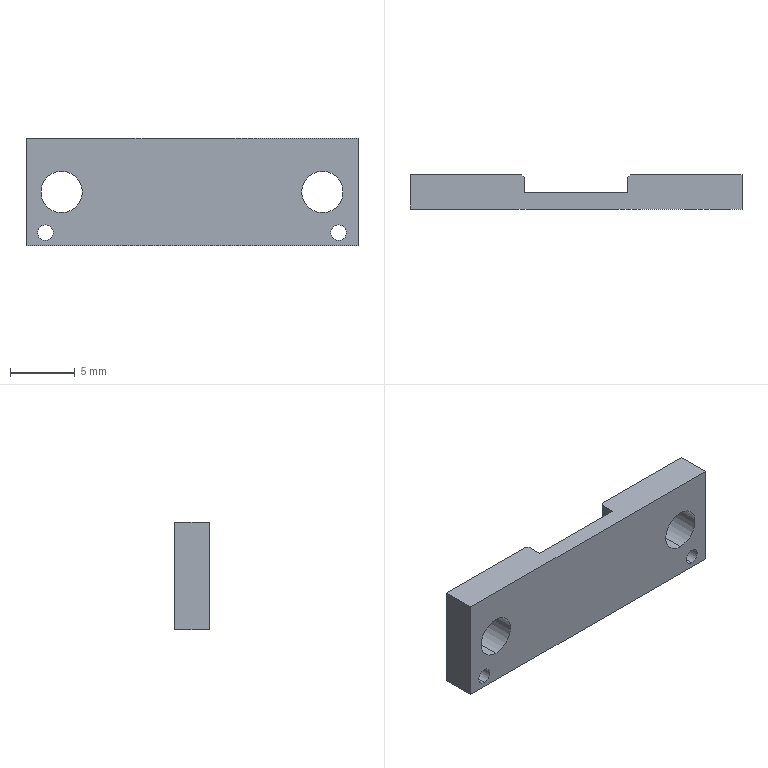Part | SolidWorks | features Chamfer 1, Extrusion 1, ICE 1 | 1 solid | 20 faces | box 25.7 x 2.65 x 8.3 mm | volume 426.68 mm3 | plane 12 | cylinder 8 | commonest cylinder face diameters 1.2 x4 3.2 x4
STEP:
#1=CARTESIAN_POINT('',(10.1,2.65,-1.6));
#2=VERTEX_POINT('',#1);
#3=CARTESIAN_POINT('',(10.1,2.65,1.6));
#4=VERTEX_POINT('',#3);
#5=CARTESIAN_POINT('',(10.1,2.65,0.));
#6=DIRECTION('',(0.,1.,0.));
#7=DIRECTION('',(0.,0.,-1.));
#8=AXIS2_PLACEMENT_3D('',#5,#6,#7);
#9=CIRCLE('',#8,1.6);
#10=EDGE_CURVE('',#2,#4,#9,.T.);
#11=ORIENTED_EDGE('',*,*,#10,.T.);
#12=CARTESIAN_POINT('',(10.1,0.,1.6));
#13=VERTEX_POINT('',#12);
#14=CARTESIAN_POINT('',(10.1,2.65,1.6));
#15=DIRECTION('',(0.,-1.,0.));
#16=VECTOR('',#15,1000.);
#17=LINE('',#14,#16);
#18=EDGE_CURVE('',#4,#13,#17,.T.);
#19=ORIENTED_EDGE('',*,*,#18,.T.);
#20=CARTESIAN_POINT('',(10.1,0.,-1.6));
#21=VERTEX_POINT('',#20);
#22=CARTESIAN_POINT('',(10.1,0.,0.));
#23=DIRECTION('',(0.,1.,0.));
#24=DIRECTION('',(0.,0.,-1.));
#25=AXIS2_PLACEMENT_3D('',#22,#23,#24);
#26=CIRCLE('',#25,1.6);
#27=EDGE_CURVE('',#21,#13,#26,.T.);
#28=ORIENTED_EDGE('',*,*,#27,.F.);
#29=CARTESIAN_POINT('',(10.1,2.65,-1.6));
#30=DIRECTION('',(0.,-1.,0.));
#31=VECTOR('',#30,1000.);
#32=LINE('',#29,#31);
#33=EDGE_CURVE('',#2,#21,#32,.T.);
#34=ORIENTED_EDGE('',*,*,#33,.F.);
#35=EDGE_LOOP('',(#11,#19,#28,#34));
#36=FACE_OUTER_BOUND('',#35,.T.);
#37=CARTESIAN_POINT('',(10.1,2.65,0.));
#38=DIRECTION('',(0.,-1.,0.));
#39=DIRECTION('',(0.,0.,-1.));
#40=AXIS2_PLACEMENT_3D('',#37,#38,#39);
#41=CYLINDRICAL_SURFACE('',#40,1.6);
#42=ADVANCED_FACE('',(#36),#41,.F.);
#43=CARTESIAN_POINT('',(11.35,2.65,-3.75));
#44=VERTEX_POINT('',#43);
#45=CARTESIAN_POINT('',(11.35,2.65,-2.55));
#46=VERTEX_POINT('',#45);
#47=CARTESIAN_POINT('',(11.35,2.65,-3.15));
#48=DIRECTION('',(0.,1.,0.));
#49=DIRECTION('',(0.,0.,-1.));
#50=AXIS2_PLACEMENT_3D('',#47,#48,#49);
#51=CIRCLE('',#50,0.6);
#52=EDGE_CURVE('',#44,#46,#51,.T.);
#53=ORIENTED_EDGE('',*,*,#52,.T.);
#54=CARTESIAN_POINT('',(11.35,0.,-2.55));
#55=VERTEX_POINT('',#54);
#56=CARTESIAN_POINT('',(11.35,2.65,-2.55));
#57=DIRECTION('',(0.,-1.,0.));
#58=VECTOR('',#57,1000.);
#59=LINE('',#56,#58);
#60=EDGE_CURVE('',#46,#55,#59,.T.);
#61=ORIENTED_EDGE('',*,*,#60,.T.);
#62=CARTESIAN_POINT('',(11.35,0.,-3.75));
#63=VERTEX_POINT('',#62);
#64=CARTESIAN_POINT('',(11.35,0.,-3.15));
#65=DIRECTION('',(0.,1.,0.));
#66=DIRECTION('',(0.,0.,-1.));
#67=AXIS2_PLACEMENT_3D('',#64,#65,#66);
#68=CIRCLE('',#67,0.6);
#69=EDGE_CURVE('',#63,#55,#68,.T.);
#70=ORIENTED_EDGE('',*,*,#69,.F.);
#71=CARTESIAN_POINT('',(11.35,2.65,-3.75));
#72=DIRECTION('',(0.,-1.,0.));
#73=VECTOR('',#72,1000.);
#74=LINE('',#71,#73);
#75=EDGE_CURVE('',#44,#63,#74,.T.);
#76=ORIENTED_EDGE('',*,*,#75,.F.);
#77=EDGE_LOOP('',(#53,#61,#70,#76));
#78=FACE_OUTER_BOUND('',#77,.T.);
#79=CARTESIAN_POINT('',(11.35,2.65,-3.15));
#80=DIRECTION('',(0.,-1.,0.));
#81=DIRECTION('',(0.,0.,-1.));
#82=AXIS2_PLACEMENT_3D('',#79,#80,#81);
#83=CYLINDRICAL_SURFACE('',#82,0.6);
#84=ADVANCED_FACE('',(#78),#83,.F.);
#85=CARTESIAN_POINT('',(-11.35,2.65,-3.75));
#86=VERTEX_POINT('',#85);
#87=CARTESIAN_POINT('',(-11.35,2.65,-2.55));
#88=VERTEX_POINT('',#87);
#89=CARTESIAN_POINT('',(-11.35,2.65,-3.15));
#90=DIRECTION('',(0.,1.,0.));
#91=DIRECTION('',(0.,0.,1.));
#92=AXIS2_PLACEMENT_3D('',#89,#90,#91);
#93=CIRCLE('',#92,0.6);
#94=EDGE_CURVE('',#86,#88,#93,.T.);
#95=ORIENTED_EDGE('',*,*,#94,.T.);
#96=CARTESIAN_POINT('',(-11.35,0.,-2.55));
#97=VERTEX_POINT('',#96);
#98=CARTESIAN_POINT('',(-11.35,2.65,-2.55));
#99=DIRECTION('',(0.,-1.,0.));
#100=VECTOR('',#99,1000.);
#101=LINE('',#98,#100);
#102=EDGE_CURVE('',#88,#97,#101,.T.);
#103=ORIENTED_EDGE('',*,*,#102,.T.);
#104=CARTESIAN_POINT('',(-11.35,0.,-3.75));
#105=VERTEX_POINT('',#104);
#106=CARTESIAN_POINT('',(-11.35,0.,-3.15));
#107=DIRECTION('',(0.,1.,0.));
#108=DIRECTION('',(0.,0.,1.));
#109=AXIS2_PLACEMENT_3D('',#106,#107,#108);
#110=CIRCLE('',#109,0.6);
#111=EDGE_CURVE('',#105,#97,#110,.T.);
#112=ORIENTED_EDGE('',*,*,#111,.F.);
#113=CARTESIAN_POINT('',(-11.35,2.65,-3.75));
#114=DIRECTION('',(0.,-1.,0.));
#115=VECTOR('',#114,1000.);
#116=LINE('',#113,#115);
#117=EDGE_CURVE('',#86,#105,#116,.T.);
#118=ORIENTED_EDGE('',*,*,#117,.F.);
#119=EDGE_LOOP('',(#95,#103,#112,#118));
#120=FACE_OUTER_BOUND('',#119,.T.);
#121=CARTESIAN_POINT('',(-11.35,2.65,-3.15));
#122=DIRECTION('',(0.,-1.,0.));
#123=DIRECTION('',(0.,0.,-1.));
#124=AXIS2_PLACEMENT_3D('',#121,#122,#123);
#125=CYLINDRICAL_SURFACE('',#124,0.6);
#126=ADVANCED_FACE('',(#120),#125,.F.);
#127=CARTESIAN_POINT('',(-10.1,2.65,-1.6));
#128=VERTEX_POINT('',#127);
#129=CARTESIAN_POINT('',(-10.1,2.65,1.6));
#130=VERTEX_POINT('',#129);
#131=CARTESIAN_POINT('',(-10.1,2.65,0.));
#132=DIRECTION('',(0.,1.,0.));
#133=DIRECTION('',(0.,0.,1.));
#134=AXIS2_PLACEMENT_3D('',#131,#132,#133);
#135=CIRCLE('',#134,1.6);
#136=EDGE_CURVE('',#128,#130,#135,.T.);
#137=ORIENTED_EDGE('',*,*,#136,.T.);
#138=CARTESIAN_POINT('',(-10.1,0.,1.6));
#139=VERTEX_POINT('',#138);
#140=CARTESIAN_POINT('',(-10.1,2.65,1.6));
#141=DIRECTION('',(0.,-1.,0.));
#142=VECTOR('',#141,1000.);
#143=LINE('',#140,#142);
#144=EDGE_CURVE('',#130,#139,#143,.T.);
#145=ORIENTED_EDGE('',*,*,#144,.T.);
#146=CARTESIAN_POINT('',(-10.1,0.,-1.6));
#147=VERTEX_POINT('',#146);
#148=CARTESIAN_POINT('',(-10.1,0.,0.));
#149=DIRECTION('',(0.,1.,0.));
#150=DIRECTION('',(0.,0.,1.));
#151=AXIS2_PLACEMENT_3D('',#148,#149,#150);
#152=CIRCLE('',#151,1.6);
#153=EDGE_CURVE('',#147,#139,#152,.T.);
#154=ORIENTED_EDGE('',*,*,#153,.F.);
#155=CARTESIAN_POINT('',(-10.1,2.65,-1.6));
#156=DIRECTION('',(0.,-1.,0.));
#157=VECTOR('',#156,1000.);
#158=LINE('',#155,#157);
#159=EDGE_CURVE('',#128,#147,#158,.T.);
#160=ORIENTED_EDGE('',*,*,#159,.F.);
#161=EDGE_LOOP('',(#137,#145,#154,#160));
#162=FACE_OUTER_BOUND('',#161,.T.);
#163=CARTESIAN_POINT('',(-10.1,2.65,0.));
#164=DIRECTION('',(0.,-1.,0.));
#165=DIRECTION('',(0.,0.,-1.));
#166=AXIS2_PLACEMENT_3D('',#163,#164,#165);
#167=CYLINDRICAL_SURFACE('',#166,1.6);
#168=ADVANCED_FACE('',(#162),#167,.F.);
#169=CARTESIAN_POINT('',(12.85,2.65,-4.15));
#170=VERTEX_POINT('',#169);
#171=CARTESIAN_POINT('',(4.2,2.65,-4.15));
#172=VERTEX_POINT('',#171);
#173=CARTESIAN_POINT('',(-12.85,2.65,-4.15));
#174=DIRECTION('',(-1.,0.,0.));
#175=VECTOR('',#174,1000.);
#176=LINE('',#173,#175);
#177=EDGE_CURVE('',#170,#172,#176,.T.);
#178=ORIENTED_EDGE('',*,*,#177,.T.);
#179=CARTESIAN_POINT('',(4.2,2.65,4.15));
#180=VERTEX_POINT('',#179);
#181=CARTESIAN_POINT('',(4.2,2.65,4.15));
#182=DIRECTION('',(0.,0.,1.));
#183=VECTOR('',#182,1000.);
#184=LINE('',#181,#183);
#185=EDGE_CURVE('',#172,#180,#184,.T.);
#186=ORIENTED_EDGE('',*,*,#185,.T.);
#187=CARTESIAN_POINT('',(12.85,2.65,4.15));
#188=VERTEX_POINT('',#187);
#189=CARTESIAN_POINT('',(-12.85,2.65,4.15));
#190=DIRECTION('',(1.,0.,0.));
#191=VECTOR('',#190,1000.);
#192=LINE('',#189,#191);
#193=EDGE_CURVE('',#180,#188,#192,.T.);
#194=ORIENTED_EDGE('',*,*,#193,.T.);
#195=CARTESIAN_POINT('',(12.85,2.65,-4.15));
#196=DIRECTION('',(0.,0.,-1.));
#197=VECTOR('',#196,1000.);
#198=LINE('',#195,#197);
#199=EDGE_CURVE('',#188,#170,#198,.T.);
#200=ORIENTED_EDGE('',*,*,#199,.T.);
#201=EDGE_LOOP('',(#178,#186,#194,#200));
#202=FACE_OUTER_BOUND('',#201,.T.);
#203=ORIENTED_EDGE('',*,*,#10,.F.);
#204=CARTESIAN_POINT('',(10.1,2.65,0.));
#205=DIRECTION('',(0.,1.,0.));
#206=DIRECTION('',(0.,0.,-1.));
#207=AXIS2_PLACEMENT_3D('',#204,#205,#206);
#208=CIRCLE('',#207,1.6);
#209=EDGE_CURVE('',#4,#2,#208,.T.);
#210=ORIENTED_EDGE('',*,*,#209,.F.);
#211=EDGE_LOOP('',(#203,#210));
#212=FACE_BOUND('',#211,.T.);
#213=ORIENTED_EDGE('',*,*,#52,.F.);
#214=CARTESIAN_POINT('',(11.35,2.65,-3.15));
#215=DIRECTION('',(0.,1.,0.));
#216=DIRECTION('',(0.,0.,-1.));
#217=AXIS2_PLACEMENT_3D('',#214,#215,#216);
#218=CIRCLE('',#217,0.6);
#219=EDGE_CURVE('',#46,#44,#218,.T.);
#220=ORIENTED_EDGE('',*,*,#219,.F.);
#221=EDGE_LOOP('',(#213,#220));
#222=FACE_BOUND('',#221,.T.);
#223=CARTESIAN_POINT('',(0.,2.65,0.));
#224=DIRECTION('',(0.,1.,0.));
#225=DIRECTION('',(0.,0.,1.));
#226=AXIS2_PLACEMENT_3D('',#223,#224,#225);
#227=PLANE('',#226);
#228=ADVANCED_FACE('',(#202,#212,#222),#227,.T.);
#229=CARTESIAN_POINT('',(-12.85,2.65,4.15));
#230=VERTEX_POINT('',#229);
#231=CARTESIAN_POINT('',(-4.2,2.65,4.15));
#232=VERTEX_POINT('',#231);
#233=CARTESIAN_POINT('',(-12.85,2.65,4.15));
#234=DIRECTION('',(1.,0.,0.));
#235=VECTOR('',#234,1000.);
#236=LINE('',#233,#235);
#237=EDGE_CURVE('',#230,#232,#236,.T.);
#238=ORIENTED_EDGE('',*,*,#237,.T.);
#239=CARTESIAN_POINT('',(-4.2,2.65,-4.15));
#240=VERTEX_POINT('',#239);
#241=CARTESIAN_POINT('',(-4.2,2.65,-4.15));
#242=DIRECTION('',(0.,0.,-1.));
#243=VECTOR('',#242,1000.);
#244=LINE('',#241,#243);
#245=EDGE_CURVE('',#232,#240,#244,.T.);
#246=ORIENTED_EDGE('',*,*,#245,.T.);
#247=CARTESIAN_POINT('',(-12.85,2.65,-4.15));
#248=VERTEX_POINT('',#247);
#249=CARTESIAN_POINT('',(-12.85,2.65,-4.15));
#250=DIRECTION('',(-1.,0.,0.));
#251=VECTOR('',#250,1000.);
#252=LINE('',#249,#251);
#253=EDGE_CURVE('',#240,#248,#252,.T.);
#254=ORIENTED_EDGE('',*,*,#253,.T.);
#255=CARTESIAN_POINT('',(-12.85,2.65,-4.15));
#256=DIRECTION('',(0.,0.,1.));
#257=VECTOR('',#256,1000.);
#258=LINE('',#255,#257);
#259=EDGE_CURVE('',#248,#230,#258,.T.);
#260=ORIENTED_EDGE('',*,*,#259,.T.);
#261=EDGE_LOOP('',(#238,#246,#254,#260));
#262=FACE_OUTER_BOUND('',#261,.T.);
#263=ORIENTED_EDGE('',*,*,#136,.F.);
#264=CARTESIAN_POINT('',(-10.1,2.65,0.));
#265=DIRECTION('',(0.,1.,0.));
#266=DIRECTION('',(0.,0.,1.));
#267=AXIS2_PLACEMENT_3D('',#264,#265,#266);
#268=CIRCLE('',#267,1.6);
#269=EDGE_CURVE('',#130,#128,#268,.T.);
#270=ORIENTED_EDGE('',*,*,#269,.F.);
#271=EDGE_LOOP('',(#263,#270));
#272=FACE_BOUND('',#271,.T.);
#273=ORIENTED_EDGE('',*,*,#94,.F.);
#274=CARTESIAN_POINT('',(-11.35,2.65,-3.15));
#275=DIRECTION('',(0.,1.,0.));
#276=DIRECTION('',(0.,0.,1.));
#277=AXIS2_PLACEMENT_3D('',#274,#275,#276);
#278=CIRCLE('',#277,0.6);
#279=EDGE_CURVE('',#88,#86,#278,.T.);
#280=ORIENTED_EDGE('',*,*,#279,.F.);
#281=EDGE_LOOP('',(#273,#280));
#282=FACE_BOUND('',#281,.T.);
#283=CARTESIAN_POINT('',(0.,2.65,0.));
#284=DIRECTION('',(0.,1.,0.));
#285=DIRECTION('',(0.,0.,1.));
#286=AXIS2_PLACEMENT_3D('',#283,#284,#285);
#287=PLANE('',#286);
#288=ADVANCED_FACE('',(#262,#272,#282),#287,.T.);
#289=ORIENTED_EDGE('',*,*,#69,.T.);
#290=CARTESIAN_POINT('',(11.35,0.,-3.15));
#291=DIRECTION('',(0.,1.,0.));
#292=DIRECTION('',(0.,0.,-1.));
#293=AXIS2_PLACEMENT_3D('',#290,#291,#292);
#294=CIRCLE('',#293,0.6);
#295=EDGE_CURVE('',#55,#63,#294,.T.);
#296=ORIENTED_EDGE('',*,*,#295,.T.);
#297=EDGE_LOOP('',(#289,#296));
#298=FACE_BOUND('',#297,.T.);
#299=ORIENTED_EDGE('',*,*,#153,.T.);
#300=CARTESIAN_POINT('',(-10.1,0.,0.));
#301=DIRECTION('',(0.,1.,0.));
#302=DIRECTION('',(0.,0.,1.));
#303=AXIS2_PLACEMENT_3D('',#300,#301,#302);
#304=CIRCLE('',#303,1.6);
#305=EDGE_CURVE('',#139,#147,#304,.T.);
#306=ORIENTED_EDGE('',*,*,#305,.T.);
#307=EDGE_LOOP('',(#299,#306));
#308=FACE_BOUND('',#307,.T.);
#309=CARTESIAN_POINT('',(12.85,0.,4.15));
#310=VERTEX_POINT('',#309);
#311=CARTESIAN_POINT('',(12.85,0.,-4.15));
#312=VERTEX_POINT('',#311);
#313=CARTESIAN_POINT('',(12.85,0.,-4.15));
#314=DIRECTION('',(0.,0.,-1.));
#315=VECTOR('',#314,1000.);
#316=LINE('',#313,#315);
#317=EDGE_CURVE('',#310,#312,#316,.T.);
#318=ORIENTED_EDGE('',*,*,#317,.F.);
#319=CARTESIAN_POINT('',(-12.85,0.,4.15));
#320=VERTEX_POINT('',#319);
#321=CARTESIAN_POINT('',(-12.85,0.,4.15));
#322=DIRECTION('',(1.,0.,0.));
#323=VECTOR('',#322,1000.);
#324=LINE('',#321,#323);
#325=EDGE_CURVE('',#320,#310,#324,.T.);
#326=ORIENTED_EDGE('',*,*,#325,.F.);
#327=CARTESIAN_POINT('',(-12.85,0.,-4.15));
#328=VERTEX_POINT('',#327);
#329=CARTESIAN_POINT('',(-12.85,0.,-4.15));
#330=DIRECTION('',(0.,0.,1.));
#331=VECTOR('',#330,1000.);
#332=LINE('',#329,#331);
#333=EDGE_CURVE('',#328,#320,#332,.T.);
#334=ORIENTED_EDGE('',*,*,#333,.F.);
#335=CARTESIAN_POINT('',(-12.85,0.,-4.15));
#336=DIRECTION('',(-1.,0.,0.));
#337=VECTOR('',#336,1000.);
#338=LINE('',#335,#337);
#339=EDGE_CURVE('',#312,#328,#338,.T.);
#340=ORIENTED_EDGE('',*,*,#339,.F.);
#341=EDGE_LOOP('',(#318,#326,#334,#340));
#342=FACE_OUTER_BOUND('',#341,.T.);
#343=ORIENTED_EDGE('',*,*,#111,.T.);
#344=CARTESIAN_POINT('',(-11.35,0.,-3.15));
#345=DIRECTION('',(0.,1.,0.));
#346=DIRECTION('',(0.,0.,1.));
#347=AXIS2_PLACEMENT_3D('',#344,#345,#346);
#348=CIRCLE('',#347,0.6);
#349=EDGE_CURVE('',#97,#105,#348,.T.);
#350=ORIENTED_EDGE('',*,*,#349,.T.);
#351=EDGE_LOOP('',(#343,#350));
#352=FACE_BOUND('',#351,.T.);
#353=ORIENTED_EDGE('',*,*,#27,.T.);
#354=CARTESIAN_POINT('',(10.1,0.,0.));
#355=DIRECTION('',(0.,1.,0.));
#356=DIRECTION('',(0.,0.,-1.));
#357=AXIS2_PLACEMENT_3D('',#354,#355,#356);
#358=CIRCLE('',#357,1.6);
#359=EDGE_CURVE('',#13,#21,#358,.T.);
#360=ORIENTED_EDGE('',*,*,#359,.T.);
#361=EDGE_LOOP('',(#353,#360));
#362=FACE_BOUND('',#361,.T.);
#363=CARTESIAN_POINT('',(0.,0.,0.));
#364=DIRECTION('',(0.,1.,0.));
#365=DIRECTION('',(0.,0.,1.));
#366=AXIS2_PLACEMENT_3D('',#363,#364,#365);
#367=PLANE('',#366);
#368=ADVANCED_FACE('',(#298,#308,#342,#352,#362),#367,.F.);
#369=ORIENTED_EDGE('',*,*,#317,.T.);
#370=CARTESIAN_POINT('',(12.85,2.65,-4.15));
#371=DIRECTION('',(0.,-1.,0.));
#372=VECTOR('',#371,1000.);
#373=LINE('',#370,#372);
#374=EDGE_CURVE('',#170,#312,#373,.T.);
#375=ORIENTED_EDGE('',*,*,#374,.F.);
#376=ORIENTED_EDGE('',*,*,#199,.F.);
#377=CARTESIAN_POINT('',(12.85,2.65,4.15));
#378=DIRECTION('',(0.,-1.,0.));
#379=VECTOR('',#378,1000.);
#380=LINE('',#377,#379);
#381=EDGE_CURVE('',#188,#310,#380,.T.);
#382=ORIENTED_EDGE('',*,*,#381,.T.);
#383=EDGE_LOOP('',(#369,#375,#376,#382));
#384=FACE_OUTER_BOUND('',#383,.T.);
#385=CARTESIAN_POINT('',(12.85,2.65,-4.15));
#386=DIRECTION('',(-1.,0.,0.));
#387=DIRECTION('',(0.,0.,1.));
#388=AXIS2_PLACEMENT_3D('',#385,#386,#387);
#389=PLANE('',#388);
#390=ADVANCED_FACE('',(#384),#389,.F.);
#391=CARTESIAN_POINT('',(4.,1.3,-4.15));
#392=VERTEX_POINT('',#391);
#393=CARTESIAN_POINT('',(4.,2.45,-4.15));
#394=VERTEX_POINT('',#393);
#395=CARTESIAN_POINT('',(4.,1.3,-4.15));
#396=DIRECTION('',(0.,1.,0.));
#397=VECTOR('',#396,1000.);
#398=LINE('',#395,#397);
#399=EDGE_CURVE('',#392,#394,#398,.T.);
#400=ORIENTED_EDGE('',*,*,#399,.T.);
#401=CARTESIAN_POINT('',(4.,2.45,-4.15));
#402=DIRECTION('',(0.7071,0.7071,0.));
#403=VECTOR('',#402,1000.);
#404=LINE('',#401,#403);
#405=EDGE_CURVE('',#394,#172,#404,.T.);
#406=ORIENTED_EDGE('',*,*,#405,.T.);
#407=ORIENTED_EDGE('',*,*,#177,.F.);
#408=ORIENTED_EDGE('',*,*,#374,.T.);
#409=ORIENTED_EDGE('',*,*,#339,.T.);
#410=CARTESIAN_POINT('',(-12.85,2.65,-4.15));
#411=DIRECTION('',(0.,-1.,0.));
#412=VECTOR('',#411,1000.);
#413=LINE('',#410,#412);
#414=EDGE_CURVE('',#248,#328,#413,.T.);
#415=ORIENTED_EDGE('',*,*,#414,.F.);
#416=ORIENTED_EDGE('',*,*,#253,.F.);
#417=CARTESIAN_POINT('',(-4.,2.45,-4.15));
#418=VERTEX_POINT('',#417);
#419=CARTESIAN_POINT('',(-4.,2.45,-4.15));
#420=DIRECTION('',(0.7071,-0.7071,0.));
#421=VECTOR('',#420,1000.);
#422=LINE('',#419,#421);
#423=EDGE_CURVE('',#240,#418,#422,.T.);
#424=ORIENTED_EDGE('',*,*,#423,.T.);
#425=CARTESIAN_POINT('',(-4.,1.3,-4.15));
#426=VERTEX_POINT('',#425);
#427=CARTESIAN_POINT('',(-4.,1.3,-4.15));
#428=DIRECTION('',(0.,1.,0.));
#429=VECTOR('',#428,1000.);
#430=LINE('',#427,#429);
#431=EDGE_CURVE('',#426,#418,#430,.T.);
#432=ORIENTED_EDGE('',*,*,#431,.F.);
#433=CARTESIAN_POINT('',(-4.,1.3,-4.15));
#434=DIRECTION('',(-1.,0.,0.));
#435=VECTOR('',#434,1000.);
#436=LINE('',#433,#435);
#437=EDGE_CURVE('',#392,#426,#436,.T.);
#438=ORIENTED_EDGE('',*,*,#437,.F.);
#439=EDGE_LOOP('',(#400,#406,#407,#408,#409,#415,#416,#424,#432,#438));
#440=FACE_OUTER_BOUND('',#439,.T.);
#441=CARTESIAN_POINT('',(-12.85,2.65,-4.15));
#442=DIRECTION('',(0.,0.,1.));
#443=DIRECTION('',(1.,0.,0.));
#444=AXIS2_PLACEMENT_3D('',#441,#442,#443);
#445=PLANE('',#444);
#446=ADVANCED_FACE('',(#440),#445,.F.);
#447=ORIENTED_EDGE('',*,*,#333,.T.);
#448=CARTESIAN_POINT('',(-12.85,2.65,4.15));
#449=DIRECTION('',(0.,-1.,0.));
#450=VECTOR('',#449,1000.);
#451=LINE('',#448,#450);
#452=EDGE_CURVE('',#230,#320,#451,.T.);
#453=ORIENTED_EDGE('',*,*,#452,.F.);
#454=ORIENTED_EDGE('',*,*,#259,.F.);
#455=ORIENTED_EDGE('',*,*,#414,.T.);
#456=EDGE_LOOP('',(#447,#453,#454,#455));
#457=FACE_OUTER_BOUND('',#456,.T.);
#458=CARTESIAN_POINT('',(-12.85,2.65,-4.15));
#459=DIRECTION('',(1.,0.,0.));
#460=DIRECTION('',(0.,0.,-1.));
#461=AXIS2_PLACEMENT_3D('',#458,#459,#460);
#462=PLANE('',#461);
#463=ADVANCED_FACE('',(#457),#462,.F.);
#464=ORIENTED_EDGE('',*,*,#193,.F.);
#465=CARTESIAN_POINT('',(4.,2.45,4.15));
#466=VERTEX_POINT('',#465);
#467=CARTESIAN_POINT('',(4.,2.45,4.15));
#468=DIRECTION('',(-0.7071,-0.7071,0.));
#469=VECTOR('',#468,1000.);
#470=LINE('',#467,#469);
#471=EDGE_CURVE('',#180,#466,#470,.T.);
#472=ORIENTED_EDGE('',*,*,#471,.T.);
#473=CARTESIAN_POINT('',(4.,1.3,4.15));
#474=VERTEX_POINT('',#473);
#475=CARTESIAN_POINT('',(4.,1.3,4.15));
#476=DIRECTION('',(0.,1.,0.));
#477=VECTOR('',#476,1000.);
#478=LINE('',#475,#477);
#479=EDGE_CURVE('',#474,#466,#478,.T.);
#480=ORIENTED_EDGE('',*,*,#479,.F.);
#481=CARTESIAN_POINT('',(-4.,1.3,4.15));
#482=VERTEX_POINT('',#481);
#483=CARTESIAN_POINT('',(-4.,1.3,4.15));
#484=DIRECTION('',(1.,0.,0.));
#485=VECTOR('',#484,1000.);
#486=LINE('',#483,#485);
#487=EDGE_CURVE('',#482,#474,#486,.T.);
#488=ORIENTED_EDGE('',*,*,#487,.F.);
#489=CARTESIAN_POINT('',(-4.,2.45,4.15));
#490=VERTEX_POINT('',#489);
#491=CARTESIAN_POINT('',(-4.,1.3,4.15));
#492=DIRECTION('',(0.,1.,0.));
#493=VECTOR('',#492,1000.);
#494=LINE('',#491,#493);
#495=EDGE_CURVE('',#482,#490,#494,.T.);
#496=ORIENTED_EDGE('',*,*,#495,.T.);
#497=CARTESIAN_POINT('',(-4.,2.45,4.15));
#498=DIRECTION('',(-0.7071,0.7071,0.));
#499=VECTOR('',#498,1000.);
#500=LINE('',#497,#499);
#501=EDGE_CURVE('',#490,#232,#500,.T.);
#502=ORIENTED_EDGE('',*,*,#501,.T.);
#503=ORIENTED_EDGE('',*,*,#237,.F.);
#504=ORIENTED_EDGE('',*,*,#452,.T.);
#505=ORIENTED_EDGE('',*,*,#325,.T.);
#506=ORIENTED_EDGE('',*,*,#381,.F.);
#507=EDGE_LOOP('',(#464,#472,#480,#488,#496,#502,#503,#504,#505,#506));
#508=FACE_OUTER_BOUND('',#507,.T.);
#509=CARTESIAN_POINT('',(-12.85,2.65,4.15));
#510=DIRECTION('',(0.,0.,-1.));
#511=DIRECTION('',(-1.,0.,0.));
#512=AXIS2_PLACEMENT_3D('',#509,#510,#511);
#513=PLANE('',#512);
#514=ADVANCED_FACE('',(#508),#513,.F.);
#515=ORIENTED_EDGE('',*,*,#144,.F.);
#516=ORIENTED_EDGE('',*,*,#269,.T.);
#517=ORIENTED_EDGE('',*,*,#159,.T.);
#518=ORIENTED_EDGE('',*,*,#305,.F.);
#519=EDGE_LOOP('',(#515,#516,#517,#518));
#520=FACE_OUTER_BOUND('',#519,.T.);
#521=CARTESIAN_POINT('',(-10.1,2.65,0.));
#522=DIRECTION('',(0.,-1.,0.));
#523=DIRECTION('',(0.,0.,-1.));
#524=AXIS2_PLACEMENT_3D('',#521,#522,#523);
#525=CYLINDRICAL_SURFACE('',#524,1.6);
#526=ADVANCED_FACE('',(#520),#525,.F.);
#527=ORIENTED_EDGE('',*,*,#102,.F.);
#528=ORIENTED_EDGE('',*,*,#279,.T.);
#529=ORIENTED_EDGE('',*,*,#117,.T.);
#530=ORIENTED_EDGE('',*,*,#349,.F.);
#531=EDGE_LOOP('',(#527,#528,#529,#530));
#532=FACE_OUTER_BOUND('',#531,.T.);
#533=CARTESIAN_POINT('',(-11.35,2.65,-3.15));
#534=DIRECTION('',(0.,-1.,0.));
#535=DIRECTION('',(0.,0.,-1.));
#536=AXIS2_PLACEMENT_3D('',#533,#534,#535);
#537=CYLINDRICAL_SURFACE('',#536,0.6);
#538=ADVANCED_FACE('',(#532),#537,.F.);
#539=ORIENTED_EDGE('',*,*,#60,.F.);
#540=ORIENTED_EDGE('',*,*,#219,.T.);
#541=ORIENTED_EDGE('',*,*,#75,.T.);
#542=ORIENTED_EDGE('',*,*,#295,.F.);
#543=EDGE_LOOP('',(#539,#540,#541,#542));
#544=FACE_OUTER_BOUND('',#543,.T.);
#545=CARTESIAN_POINT('',(11.35,2.65,-3.15));
#546=DIRECTION('',(0.,-1.,0.));
#547=DIRECTION('',(0.,0.,-1.));
#548=AXIS2_PLACEMENT_3D('',#545,#546,#547);
#549=CYLINDRICAL_SURFACE('',#548,0.6);
#550=ADVANCED_FACE('',(#544),#549,.F.);
#551=ORIENTED_EDGE('',*,*,#18,.F.);
#552=ORIENTED_EDGE('',*,*,#209,.T.);
#553=ORIENTED_EDGE('',*,*,#33,.T.);
#554=ORIENTED_EDGE('',*,*,#359,.F.);
#555=EDGE_LOOP('',(#551,#552,#553,#554));
#556=FACE_OUTER_BOUND('',#555,.T.);
#557=CARTESIAN_POINT('',(10.1,2.65,0.));
#558=DIRECTION('',(0.,-1.,0.));
#559=DIRECTION('',(0.,0.,-1.));
#560=AXIS2_PLACEMENT_3D('',#557,#558,#559);
#561=CYLINDRICAL_SURFACE('',#560,1.6);
#562=ADVANCED_FACE('',(#556),#561,.F.);
#563=ORIENTED_EDGE('',*,*,#479,.T.);
#564=CARTESIAN_POINT('',(4.,2.45,-4.15));
#565=DIRECTION('',(0.,0.,-1.));
#566=VECTOR('',#565,1000.);
#567=LINE('',#564,#566);
#568=EDGE_CURVE('',#466,#394,#567,.T.);
#569=ORIENTED_EDGE('',*,*,#568,.T.);
#570=ORIENTED_EDGE('',*,*,#399,.F.);
#571=CARTESIAN_POINT('',(4.,1.3,-4.15));
#572=DIRECTION('',(0.,0.,-1.));
#573=VECTOR('',#572,1000.);
#574=LINE('',#571,#573);
#575=EDGE_CURVE('',#474,#392,#574,.T.);
#576=ORIENTED_EDGE('',*,*,#575,.F.);
#577=EDGE_LOOP('',(#563,#569,#570,#576));
#578=FACE_OUTER_BOUND('',#577,.T.);
#579=CARTESIAN_POINT('',(4.,1.3,-4.15));
#580=DIRECTION('',(1.,0.,0.));
#581=DIRECTION('',(0.,0.,-1.));
#582=AXIS2_PLACEMENT_3D('',#579,#580,#581);
#583=PLANE('',#582);
#584=ADVANCED_FACE('',(#578),#583,.F.);
#585=ORIENTED_EDGE('',*,*,#431,.T.);
#586=CARTESIAN_POINT('',(-4.,2.45,4.15));
#587=DIRECTION('',(0.,0.,1.));
#588=VECTOR('',#587,1000.);
#589=LINE('',#586,#588);
#590=EDGE_CURVE('',#418,#490,#589,.T.);
#591=ORIENTED_EDGE('',*,*,#590,.T.);
#592=ORIENTED_EDGE('',*,*,#495,.F.);
#593=CARTESIAN_POINT('',(-4.,1.3,-4.15));
#594=DIRECTION('',(0.,0.,1.));
#595=VECTOR('',#594,1000.);
#596=LINE('',#593,#595);
#597=EDGE_CURVE('',#426,#482,#596,.T.);
#598=ORIENTED_EDGE('',*,*,#597,.F.);
#599=EDGE_LOOP('',(#585,#591,#592,#598));
#600=FACE_OUTER_BOUND('',#599,.T.);
#601=CARTESIAN_POINT('',(-4.,1.3,-4.15));
#602=DIRECTION('',(-1.,0.,0.));
#603=DIRECTION('',(0.,0.,1.));
#604=AXIS2_PLACEMENT_3D('',#601,#602,#603);
#605=PLANE('',#604);
#606=ADVANCED_FACE('',(#600),#605,.F.);
#607=ORIENTED_EDGE('',*,*,#575,.T.);
#608=ORIENTED_EDGE('',*,*,#437,.T.);
#609=ORIENTED_EDGE('',*,*,#597,.T.);
#610=ORIENTED_EDGE('',*,*,#487,.T.);
#611=EDGE_LOOP('',(#607,#608,#609,#610));
#612=FACE_OUTER_BOUND('',#611,.T.);
#613=CARTESIAN_POINT('',(0.,1.3,0.));
#614=DIRECTION('',(0.,1.,0.));
#615=DIRECTION('',(0.,0.,1.));
#616=AXIS2_PLACEMENT_3D('',#613,#614,#615);
#617=PLANE('',#616);
#618=ADVANCED_FACE('',(#612),#617,.T.);
#619=ORIENTED_EDGE('',*,*,#471,.F.);
#620=ORIENTED_EDGE('',*,*,#185,.F.);
#621=ORIENTED_EDGE('',*,*,#405,.F.);
#622=ORIENTED_EDGE('',*,*,#568,.F.);
#623=EDGE_LOOP('',(#619,#620,#621,#622));
#624=FACE_OUTER_BOUND('',#623,.T.);
#625=CARTESIAN_POINT('',(4.,2.45,-4.15));
#626=DIRECTION('',(-0.7071,0.7071,0.));
#627=DIRECTION('',(0.,0.,1.));
#628=AXIS2_PLACEMENT_3D('',#625,#626,#627);
#629=PLANE('',#628);
#630=ADVANCED_FACE('',(#624),#629,.T.);
#631=ORIENTED_EDGE('',*,*,#423,.F.);
#632=ORIENTED_EDGE('',*,*,#245,.F.);
#633=ORIENTED_EDGE('',*,*,#501,.F.);
#634=ORIENTED_EDGE('',*,*,#590,.F.);
#635=EDGE_LOOP('',(#631,#632,#633,#634));
#636=FACE_OUTER_BOUND('',#635,.T.);
#637=CARTESIAN_POINT('',(-4.,2.45,-4.15));
#638=DIRECTION('',(0.7071,0.7071,0.));
#639=DIRECTION('',(0.,0.,-1.));
#640=AXIS2_PLACEMENT_3D('',#637,#638,#639);
#641=PLANE('',#640);
#642=ADVANCED_FACE('',(#636),#641,.T.);
#643=CLOSED_SHELL('',(#42,#84,#126,#168,#228,#288,#368,#390,#446,#463,#514,#526,#538,#550,#562,#584,#606,#618,#630,#642));
#644=MANIFOLD_SOLID_BREP('',#643);
#645=CARTESIAN_POINT('',(0.,0.,0.));
#646=DIRECTION('',(0.,0.,1.));
#647=DIRECTION('',(1.,0.,0.));
#648=AXIS2_PLACEMENT_3D('',#645,#646,#647);
#649=(LENGTH_UNIT()NAMED_UNIT(*)SI_UNIT(.MILLI.,.METRE.));
#650=UNCERTAINTY_MEASURE_WITH_UNIT(LENGTH_MEASURE(0.00001),#649,'','');
#651=(NAMED_UNIT(*)PLANE_ANGLE_UNIT()SI_UNIT($,.RADIAN.));
#652=(NAMED_UNIT(*)SI_UNIT($,.STERADIAN.)SOLID_ANGLE_UNIT());
#653=(GEOMETRIC_REPRESENTATION_CONTEXT(3)GLOBAL_UNCERTAINTY_ASSIGNED_CONTEXT((#650))GLOBAL_UNIT_ASSIGNED_CONTEXT((#649,#651,#652))REPRESENTATION_CONTEXT('',''));
#654=ADVANCED_BREP_SHAPE_REPRESENTATION('',(#644,#648),#653);